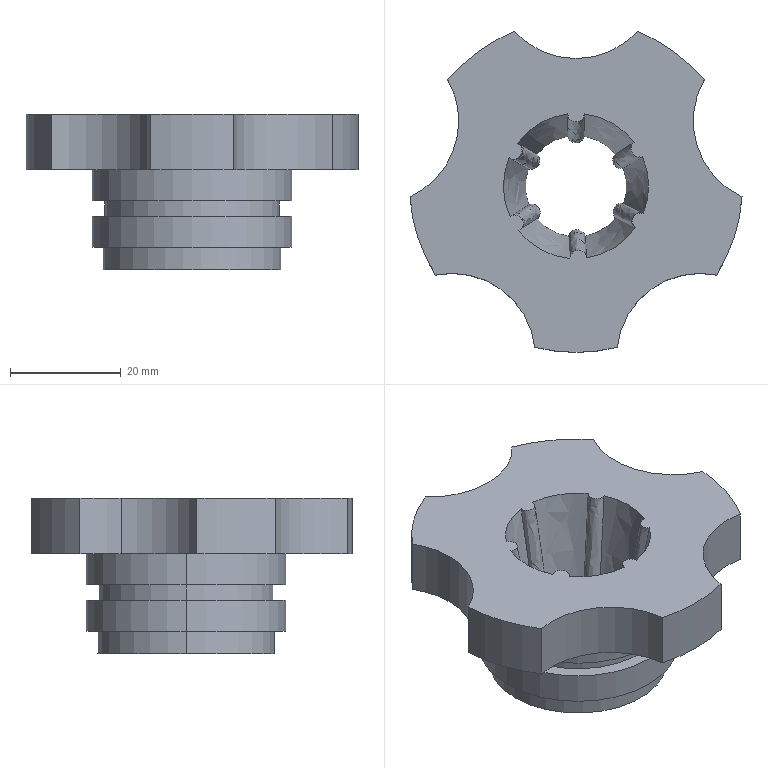Part | STEP file | Adjusting nut SGN-4-09-01 (9) | 1 solid | 51 faces | box 59.878 x 57.882 x 28 mm | volume 29055 mm3 | spline 24 | cylinder 19 | plane 6 | cone 2 | commonest cylinder face diameters 30 x6 60 x5 36 x4 31.5 x2 32 x2